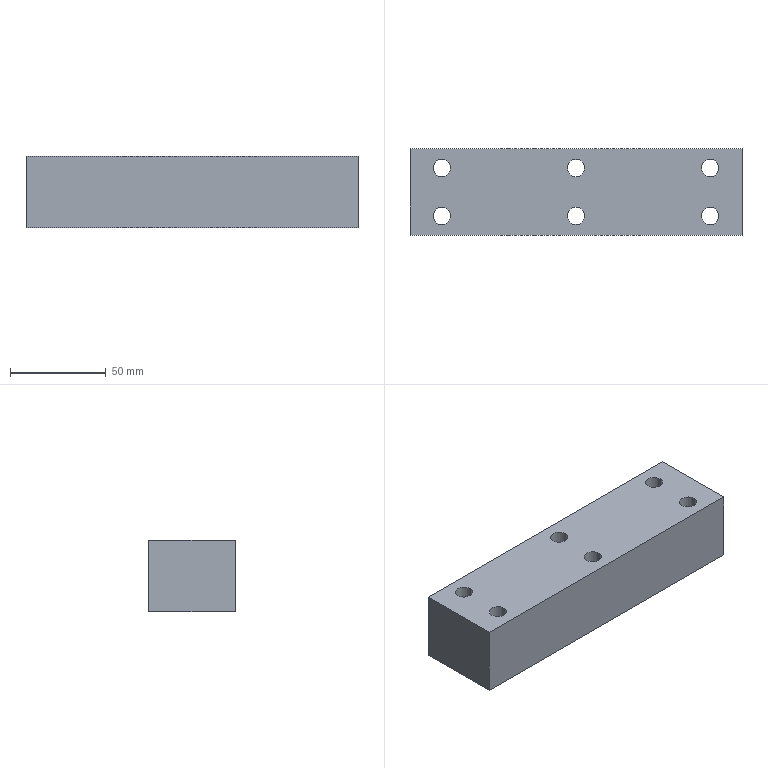Part | STEP file | 44-02-16 Press-fit Connecting Plate | 1 solid | 18 faces | box 173 x 45 x 37 mm | volume 273922 mm3 | cylinder 12 | plane 6 | commonest cylinder face diameters 9 x12
STEP:
#1=CARTESIAN_POINT('',(0.,0.,0.));
#2=DIRECTION('',(0.,0.,1.));
#3=DIRECTION('',(1.,0.,0.));
#4=AXIS2_PLACEMENT_3D('',#1,#2,#3);
#5=CARTESIAN_POINT('',(4.5,12.5,-18.5));
#6=VERTEX_POINT('',#5);
#7=CARTESIAN_POINT('',(4.5,12.5,18.5));
#8=VERTEX_POINT('',#7);
#9=CARTESIAN_POINT('',(4.5,12.5,-18.5));
#10=DIRECTION('',(0.,0.,1.));
#11=VECTOR('',#10,1.);
#12=LINE('',#9,#11);
#13=CARTESIAN_POINT('',(0.,12.5,-18.5));
#14=DIRECTION('',(0.,0.,1.));
#15=DIRECTION('',(1.,0.,0.));
#16=AXIS2_PLACEMENT_3D('',#13,#14,#15);
#17=CYLINDRICAL_SURFACE('',#16,4.5);
#18=CARTESIAN_POINT('',(6.283,0.));
#19=DIRECTION('',(0.,1.));
#20=VECTOR('',#19,1.);
#21=LINE('',#18,#20);
#22=(GEOMETRIC_REPRESENTATION_CONTEXT(2)PARAMETRIC_REPRESENTATION_CONTEXT()REPRESENTATION_CONTEXT('',''));
#23=DEFINITIONAL_REPRESENTATION('',(#21),#22);
#24=PCURVE('',#17,#23);
#25=CARTESIAN_POINT('',(0.,12.5,-18.5));
#26=DIRECTION('',(0.,0.,1.));
#27=DIRECTION('',(1.,0.,0.));
#28=AXIS2_PLACEMENT_3D('',#25,#26,#27);
#29=CYLINDRICAL_SURFACE('',#28,4.5);
#30=CARTESIAN_POINT('',(0.,0.));
#31=DIRECTION('',(0.,1.));
#32=VECTOR('',#31,1.);
#33=LINE('',#30,#32);
#34=(GEOMETRIC_REPRESENTATION_CONTEXT(2)PARAMETRIC_REPRESENTATION_CONTEXT()REPRESENTATION_CONTEXT('',''));
#35=DEFINITIONAL_REPRESENTATION('',(#33),#34);
#36=PCURVE('',#29,#35);
#37=SURFACE_CURVE('',#12,(#24,#36),.PCURVE_S1.);
#38=EDGE_CURVE('',#6,#8,#37,.T.);
#39=ORIENTED_EDGE('',*,*,#38,.T.);
#40=CARTESIAN_POINT('',(-4.5,12.5,18.5));
#41=VERTEX_POINT('',#40);
#42=CARTESIAN_POINT('',(0.,12.5,18.5));
#43=DIRECTION('',(0.,0.,1.));
#44=DIRECTION('',(1.,0.,0.));
#45=AXIS2_PLACEMENT_3D('',#42,#43,#44);
#46=CIRCLE('',#45,4.5);
#47=CARTESIAN_POINT('',(0.,37.));
#48=DIRECTION('',(1.,0.));
#49=VECTOR('',#48,1.);
#50=LINE('',#47,#49);
#51=(GEOMETRIC_REPRESENTATION_CONTEXT(2)PARAMETRIC_REPRESENTATION_CONTEXT()REPRESENTATION_CONTEXT('',''));
#52=DEFINITIONAL_REPRESENTATION('',(#50),#51);
#53=PCURVE('',#17,#52);
#54=CARTESIAN_POINT('',(86.5,-22.5,18.5));
#55=DIRECTION('',(0.,0.,1.));
#56=DIRECTION('',(1.,0.,0.));
#57=AXIS2_PLACEMENT_3D('',#54,#55,#56);
#58=PLANE('',#57);
#59=CARTESIAN_POINT('',(-86.5,35.));
#60=DIRECTION('',(1.,0.));
#61=AXIS2_PLACEMENT_2D('',#59,#60);
#62=CIRCLE('',#61,4.5);
#63=(GEOMETRIC_REPRESENTATION_CONTEXT(2)PARAMETRIC_REPRESENTATION_CONTEXT()REPRESENTATION_CONTEXT('',''));
#64=DEFINITIONAL_REPRESENTATION('',(#62),#63);
#65=PCURVE('',#58,#64);
#66=SURFACE_CURVE('',#46,(#53,#65),.PCURVE_S1.);
#67=EDGE_CURVE('',#41,#8,#66,.T.);
#68=ORIENTED_EDGE('',*,*,#67,.F.);
#69=CARTESIAN_POINT('',(-4.5,12.5,-18.5));
#70=VERTEX_POINT('',#69);
#71=CARTESIAN_POINT('',(-4.5,12.5,-18.5));
#72=DIRECTION('',(0.,0.,1.));
#73=VECTOR('',#72,1.);
#74=LINE('',#71,#73);
#75=CARTESIAN_POINT('',(3.142,0.));
#76=DIRECTION('',(0.,1.));
#77=VECTOR('',#76,1.);
#78=LINE('',#75,#77);
#79=(GEOMETRIC_REPRESENTATION_CONTEXT(2)PARAMETRIC_REPRESENTATION_CONTEXT()REPRESENTATION_CONTEXT('',''));
#80=DEFINITIONAL_REPRESENTATION('',(#78),#79);
#81=PCURVE('',#17,#80);
#82=CARTESIAN_POINT('',(3.142,0.));
#83=DIRECTION('',(0.,1.));
#84=VECTOR('',#83,1.);
#85=LINE('',#82,#84);
#86=(GEOMETRIC_REPRESENTATION_CONTEXT(2)PARAMETRIC_REPRESENTATION_CONTEXT()REPRESENTATION_CONTEXT('',''));
#87=DEFINITIONAL_REPRESENTATION('',(#85),#86);
#88=PCURVE('',#29,#87);
#89=SURFACE_CURVE('',#74,(#81,#88),.PCURVE_S1.);
#90=EDGE_CURVE('',#70,#41,#89,.T.);
#91=ORIENTED_EDGE('',*,*,#90,.F.);
#92=CARTESIAN_POINT('',(0.,12.5,-18.5));
#93=DIRECTION('',(0.,0.,1.));
#94=DIRECTION('',(1.,0.,0.));
#95=AXIS2_PLACEMENT_3D('',#92,#93,#94);
#96=CIRCLE('',#95,4.5);
#97=CARTESIAN_POINT('',(0.,0.));
#98=DIRECTION('',(1.,0.));
#99=VECTOR('',#98,1.);
#100=LINE('',#97,#99);
#101=(GEOMETRIC_REPRESENTATION_CONTEXT(2)PARAMETRIC_REPRESENTATION_CONTEXT()REPRESENTATION_CONTEXT('',''));
#102=DEFINITIONAL_REPRESENTATION('',(#100),#101);
#103=PCURVE('',#17,#102);
#104=CARTESIAN_POINT('',(86.5,-22.5,-18.5));
#105=DIRECTION('',(0.,0.,1.));
#106=DIRECTION('',(1.,0.,0.));
#107=AXIS2_PLACEMENT_3D('',#104,#105,#106);
#108=PLANE('',#107);
#109=CARTESIAN_POINT('',(-86.5,35.));
#110=DIRECTION('',(1.,0.));
#111=AXIS2_PLACEMENT_2D('',#109,#110);
#112=CIRCLE('',#111,4.5);
#113=(GEOMETRIC_REPRESENTATION_CONTEXT(2)PARAMETRIC_REPRESENTATION_CONTEXT()REPRESENTATION_CONTEXT('',''));
#114=DEFINITIONAL_REPRESENTATION('',(#112),#113);
#115=PCURVE('',#108,#114);
#116=SURFACE_CURVE('',#96,(#103,#115),.PCURVE_S1.);
#117=EDGE_CURVE('',#70,#6,#116,.T.);
#118=ORIENTED_EDGE('',*,*,#117,.T.);
#119=EDGE_LOOP('',(#39,#68,#91,#118));
#120=FACE_BOUND('',#119,.F.);
#121=ADVANCED_FACE('',(#120),#17,.F.);
#122=CARTESIAN_POINT('',(4.5,-12.5,-18.5));
#123=VERTEX_POINT('',#122);
#124=CARTESIAN_POINT('',(4.5,-12.5,18.5));
#125=VERTEX_POINT('',#124);
#126=CARTESIAN_POINT('',(4.5,-12.5,-18.5));
#127=DIRECTION('',(0.,0.,1.));
#128=VECTOR('',#127,1.);
#129=LINE('',#126,#128);
#130=CARTESIAN_POINT('',(0.,-12.5,-18.5));
#131=DIRECTION('',(0.,0.,1.));
#132=DIRECTION('',(1.,0.,0.));
#133=AXIS2_PLACEMENT_3D('',#130,#131,#132);
#134=CYLINDRICAL_SURFACE('',#133,4.5);
#135=CARTESIAN_POINT('',(6.283,0.));
#136=DIRECTION('',(0.,1.));
#137=VECTOR('',#136,1.);
#138=LINE('',#135,#137);
#139=(GEOMETRIC_REPRESENTATION_CONTEXT(2)PARAMETRIC_REPRESENTATION_CONTEXT()REPRESENTATION_CONTEXT('',''));
#140=DEFINITIONAL_REPRESENTATION('',(#138),#139);
#141=PCURVE('',#134,#140);
#142=CARTESIAN_POINT('',(0.,-12.5,-18.5));
#143=DIRECTION('',(0.,0.,1.));
#144=DIRECTION('',(1.,0.,0.));
#145=AXIS2_PLACEMENT_3D('',#142,#143,#144);
#146=CYLINDRICAL_SURFACE('',#145,4.5);
#147=CARTESIAN_POINT('',(0.,0.));
#148=DIRECTION('',(0.,1.));
#149=VECTOR('',#148,1.);
#150=LINE('',#147,#149);
#151=(GEOMETRIC_REPRESENTATION_CONTEXT(2)PARAMETRIC_REPRESENTATION_CONTEXT()REPRESENTATION_CONTEXT('',''));
#152=DEFINITIONAL_REPRESENTATION('',(#150),#151);
#153=PCURVE('',#146,#152);
#154=SURFACE_CURVE('',#129,(#141,#153),.PCURVE_S1.);
#155=EDGE_CURVE('',#123,#125,#154,.T.);
#156=ORIENTED_EDGE('',*,*,#155,.T.);
#157=CARTESIAN_POINT('',(-4.5,-12.5,18.5));
#158=VERTEX_POINT('',#157);
#159=CARTESIAN_POINT('',(0.,-12.5,18.5));
#160=DIRECTION('',(0.,0.,1.));
#161=DIRECTION('',(1.,0.,0.));
#162=AXIS2_PLACEMENT_3D('',#159,#160,#161);
#163=CIRCLE('',#162,4.5);
#164=CARTESIAN_POINT('',(0.,37.));
#165=DIRECTION('',(1.,0.));
#166=VECTOR('',#165,1.);
#167=LINE('',#164,#166);
#168=(GEOMETRIC_REPRESENTATION_CONTEXT(2)PARAMETRIC_REPRESENTATION_CONTEXT()REPRESENTATION_CONTEXT('',''));
#169=DEFINITIONAL_REPRESENTATION('',(#167),#168);
#170=PCURVE('',#134,#169);
#171=CARTESIAN_POINT('',(-86.5,10.));
#172=DIRECTION('',(1.,0.));
#173=AXIS2_PLACEMENT_2D('',#171,#172);
#174=CIRCLE('',#173,4.5);
#175=(GEOMETRIC_REPRESENTATION_CONTEXT(2)PARAMETRIC_REPRESENTATION_CONTEXT()REPRESENTATION_CONTEXT('',''));
#176=DEFINITIONAL_REPRESENTATION('',(#174),#175);
#177=PCURVE('',#58,#176);
#178=SURFACE_CURVE('',#163,(#170,#177),.PCURVE_S1.);
#179=EDGE_CURVE('',#158,#125,#178,.T.);
#180=ORIENTED_EDGE('',*,*,#179,.F.);
#181=CARTESIAN_POINT('',(-4.5,-12.5,-18.5));
#182=VERTEX_POINT('',#181);
#183=CARTESIAN_POINT('',(-4.5,-12.5,-18.5));
#184=DIRECTION('',(0.,0.,1.));
#185=VECTOR('',#184,1.);
#186=LINE('',#183,#185);
#187=CARTESIAN_POINT('',(3.142,0.));
#188=DIRECTION('',(0.,1.));
#189=VECTOR('',#188,1.);
#190=LINE('',#187,#189);
#191=(GEOMETRIC_REPRESENTATION_CONTEXT(2)PARAMETRIC_REPRESENTATION_CONTEXT()REPRESENTATION_CONTEXT('',''));
#192=DEFINITIONAL_REPRESENTATION('',(#190),#191);
#193=PCURVE('',#134,#192);
#194=CARTESIAN_POINT('',(3.142,0.));
#195=DIRECTION('',(0.,1.));
#196=VECTOR('',#195,1.);
#197=LINE('',#194,#196);
#198=(GEOMETRIC_REPRESENTATION_CONTEXT(2)PARAMETRIC_REPRESENTATION_CONTEXT()REPRESENTATION_CONTEXT('',''));
#199=DEFINITIONAL_REPRESENTATION('',(#197),#198);
#200=PCURVE('',#146,#199);
#201=SURFACE_CURVE('',#186,(#193,#200),.PCURVE_S1.);
#202=EDGE_CURVE('',#182,#158,#201,.T.);
#203=ORIENTED_EDGE('',*,*,#202,.F.);
#204=CARTESIAN_POINT('',(0.,-12.5,-18.5));
#205=DIRECTION('',(0.,0.,1.));
#206=DIRECTION('',(1.,0.,0.));
#207=AXIS2_PLACEMENT_3D('',#204,#205,#206);
#208=CIRCLE('',#207,4.5);
#209=CARTESIAN_POINT('',(0.,0.));
#210=DIRECTION('',(1.,0.));
#211=VECTOR('',#210,1.);
#212=LINE('',#209,#211);
#213=(GEOMETRIC_REPRESENTATION_CONTEXT(2)PARAMETRIC_REPRESENTATION_CONTEXT()REPRESENTATION_CONTEXT('',''));
#214=DEFINITIONAL_REPRESENTATION('',(#212),#213);
#215=PCURVE('',#134,#214);
#216=CARTESIAN_POINT('',(-86.5,10.));
#217=DIRECTION('',(1.,0.));
#218=AXIS2_PLACEMENT_2D('',#216,#217);
#219=CIRCLE('',#218,4.5);
#220=(GEOMETRIC_REPRESENTATION_CONTEXT(2)PARAMETRIC_REPRESENTATION_CONTEXT()REPRESENTATION_CONTEXT('',''));
#221=DEFINITIONAL_REPRESENTATION('',(#219),#220);
#222=PCURVE('',#108,#221);
#223=SURFACE_CURVE('',#208,(#215,#222),.PCURVE_S1.);
#224=EDGE_CURVE('',#182,#123,#223,.T.);
#225=ORIENTED_EDGE('',*,*,#224,.T.);
#226=EDGE_LOOP('',(#156,#180,#203,#225));
#227=FACE_BOUND('',#226,.F.);
#228=ADVANCED_FACE('',(#227),#134,.F.);
#229=CARTESIAN_POINT('',(74.5,12.5,-18.5));
#230=VERTEX_POINT('',#229);
#231=CARTESIAN_POINT('',(74.5,12.5,18.5));
#232=VERTEX_POINT('',#231);
#233=CARTESIAN_POINT('',(74.5,12.5,-18.5));
#234=DIRECTION('',(0.,0.,1.));
#235=VECTOR('',#234,1.);
#236=LINE('',#233,#235);
#237=CARTESIAN_POINT('',(70.,12.5,-18.5));
#238=DIRECTION('',(0.,0.,1.));
#239=DIRECTION('',(1.,0.,0.));
#240=AXIS2_PLACEMENT_3D('',#237,#238,#239);
#241=CYLINDRICAL_SURFACE('',#240,4.5);
#242=CARTESIAN_POINT('',(6.283,0.));
#243=DIRECTION('',(0.,1.));
#244=VECTOR('',#243,1.);
#245=LINE('',#242,#244);
#246=(GEOMETRIC_REPRESENTATION_CONTEXT(2)PARAMETRIC_REPRESENTATION_CONTEXT()REPRESENTATION_CONTEXT('',''));
#247=DEFINITIONAL_REPRESENTATION('',(#245),#246);
#248=PCURVE('',#241,#247);
#249=CARTESIAN_POINT('',(70.,12.5,-18.5));
#250=DIRECTION('',(0.,0.,1.));
#251=DIRECTION('',(1.,0.,0.));
#252=AXIS2_PLACEMENT_3D('',#249,#250,#251);
#253=CYLINDRICAL_SURFACE('',#252,4.5);
#254=CARTESIAN_POINT('',(0.,0.));
#255=DIRECTION('',(0.,1.));
#256=VECTOR('',#255,1.);
#257=LINE('',#254,#256);
#258=(GEOMETRIC_REPRESENTATION_CONTEXT(2)PARAMETRIC_REPRESENTATION_CONTEXT()REPRESENTATION_CONTEXT('',''));
#259=DEFINITIONAL_REPRESENTATION('',(#257),#258);
#260=PCURVE('',#253,#259);
#261=SURFACE_CURVE('',#236,(#248,#260),.PCURVE_S1.);
#262=EDGE_CURVE('',#230,#232,#261,.T.);
#263=ORIENTED_EDGE('',*,*,#262,.T.);
#264=CARTESIAN_POINT('',(65.5,12.5,18.5));
#265=VERTEX_POINT('',#264);
#266=CARTESIAN_POINT('',(70.,12.5,18.5));
#267=DIRECTION('',(0.,0.,1.));
#268=DIRECTION('',(1.,0.,0.));
#269=AXIS2_PLACEMENT_3D('',#266,#267,#268);
#270=CIRCLE('',#269,4.5);
#271=CARTESIAN_POINT('',(0.,37.));
#272=DIRECTION('',(1.,0.));
#273=VECTOR('',#272,1.);
#274=LINE('',#271,#273);
#275=(GEOMETRIC_REPRESENTATION_CONTEXT(2)PARAMETRIC_REPRESENTATION_CONTEXT()REPRESENTATION_CONTEXT('',''));
#276=DEFINITIONAL_REPRESENTATION('',(#274),#275);
#277=PCURVE('',#241,#276);
#278=CARTESIAN_POINT('',(-16.5,35.));
#279=DIRECTION('',(1.,0.));
#280=AXIS2_PLACEMENT_2D('',#278,#279);
#281=CIRCLE('',#280,4.5);
#282=(GEOMETRIC_REPRESENTATION_CONTEXT(2)PARAMETRIC_REPRESENTATION_CONTEXT()REPRESENTATION_CONTEXT('',''));
#283=DEFINITIONAL_REPRESENTATION('',(#281),#282);
#284=PCURVE('',#58,#283);
#285=SURFACE_CURVE('',#270,(#277,#284),.PCURVE_S1.);
#286=EDGE_CURVE('',#265,#232,#285,.T.);
#287=ORIENTED_EDGE('',*,*,#286,.F.);
#288=CARTESIAN_POINT('',(65.5,12.5,-18.5));
#289=VERTEX_POINT('',#288);
#290=CARTESIAN_POINT('',(65.5,12.5,-18.5));
#291=DIRECTION('',(0.,0.,1.));
#292=VECTOR('',#291,1.);
#293=LINE('',#290,#292);
#294=CARTESIAN_POINT('',(3.142,0.));
#295=DIRECTION('',(0.,1.));
#296=VECTOR('',#295,1.);
#297=LINE('',#294,#296);
#298=(GEOMETRIC_REPRESENTATION_CONTEXT(2)PARAMETRIC_REPRESENTATION_CONTEXT()REPRESENTATION_CONTEXT('',''));
#299=DEFINITIONAL_REPRESENTATION('',(#297),#298);
#300=PCURVE('',#241,#299);
#301=CARTESIAN_POINT('',(3.142,0.));
#302=DIRECTION('',(0.,1.));
#303=VECTOR('',#302,1.);
#304=LINE('',#301,#303);
#305=(GEOMETRIC_REPRESENTATION_CONTEXT(2)PARAMETRIC_REPRESENTATION_CONTEXT()REPRESENTATION_CONTEXT('',''));
#306=DEFINITIONAL_REPRESENTATION('',(#304),#305);
#307=PCURVE('',#253,#306);
#308=SURFACE_CURVE('',#293,(#300,#307),.PCURVE_S1.);
#309=EDGE_CURVE('',#289,#265,#308,.T.);
#310=ORIENTED_EDGE('',*,*,#309,.F.);
#311=CARTESIAN_POINT('',(70.,12.5,-18.5));
#312=DIRECTION('',(0.,0.,1.));
#313=DIRECTION('',(1.,0.,0.));
#314=AXIS2_PLACEMENT_3D('',#311,#312,#313);
#315=CIRCLE('',#314,4.5);
#316=CARTESIAN_POINT('',(0.,0.));
#317=DIRECTION('',(1.,0.));
#318=VECTOR('',#317,1.);
#319=LINE('',#316,#318);
#320=(GEOMETRIC_REPRESENTATION_CONTEXT(2)PARAMETRIC_REPRESENTATION_CONTEXT()REPRESENTATION_CONTEXT('',''));
#321=DEFINITIONAL_REPRESENTATION('',(#319),#320);
#322=PCURVE('',#241,#321);
#323=CARTESIAN_POINT('',(-16.5,35.));
#324=DIRECTION('',(1.,0.));
#325=AXIS2_PLACEMENT_2D('',#323,#324);
#326=CIRCLE('',#325,4.5);
#327=(GEOMETRIC_REPRESENTATION_CONTEXT(2)PARAMETRIC_REPRESENTATION_CONTEXT()REPRESENTATION_CONTEXT('',''));
#328=DEFINITIONAL_REPRESENTATION('',(#326),#327);
#329=PCURVE('',#108,#328);
#330=SURFACE_CURVE('',#315,(#322,#329),.PCURVE_S1.);
#331=EDGE_CURVE('',#289,#230,#330,.T.);
#332=ORIENTED_EDGE('',*,*,#331,.T.);
#333=EDGE_LOOP('',(#263,#287,#310,#332));
#334=FACE_BOUND('',#333,.F.);
#335=ADVANCED_FACE('',(#334),#241,.F.);
#336=CARTESIAN_POINT('',(74.5,-12.5,-18.5));
#337=VERTEX_POINT('',#336);
#338=CARTESIAN_POINT('',(74.5,-12.5,18.5));
#339=VERTEX_POINT('',#338);
#340=CARTESIAN_POINT('',(74.5,-12.5,-18.5));
#341=DIRECTION('',(0.,0.,1.));
#342=VECTOR('',#341,1.);
#343=LINE('',#340,#342);
#344=CARTESIAN_POINT('',(70.,-12.5,-18.5));
#345=DIRECTION('',(0.,0.,1.));
#346=DIRECTION('',(1.,0.,0.));
#347=AXIS2_PLACEMENT_3D('',#344,#345,#346);
#348=CYLINDRICAL_SURFACE('',#347,4.5);
#349=CARTESIAN_POINT('',(6.283,0.));
#350=DIRECTION('',(0.,1.));
#351=VECTOR('',#350,1.);
#352=LINE('',#349,#351);
#353=(GEOMETRIC_REPRESENTATION_CONTEXT(2)PARAMETRIC_REPRESENTATION_CONTEXT()REPRESENTATION_CONTEXT('',''));
#354=DEFINITIONAL_REPRESENTATION('',(#352),#353);
#355=PCURVE('',#348,#354);
#356=CARTESIAN_POINT('',(70.,-12.5,-18.5));
#357=DIRECTION('',(0.,0.,1.));
#358=DIRECTION('',(1.,0.,0.));
#359=AXIS2_PLACEMENT_3D('',#356,#357,#358);
#360=CYLINDRICAL_SURFACE('',#359,4.5);
#361=CARTESIAN_POINT('',(0.,0.));
#362=DIRECTION('',(0.,1.));
#363=VECTOR('',#362,1.);
#364=LINE('',#361,#363);
#365=(GEOMETRIC_REPRESENTATION_CONTEXT(2)PARAMETRIC_REPRESENTATION_CONTEXT()REPRESENTATION_CONTEXT('',''));
#366=DEFINITIONAL_REPRESENTATION('',(#364),#365);
#367=PCURVE('',#360,#366);
#368=SURFACE_CURVE('',#343,(#355,#367),.PCURVE_S1.);
#369=EDGE_CURVE('',#337,#339,#368,.T.);
#370=ORIENTED_EDGE('',*,*,#369,.T.);
#371=CARTESIAN_POINT('',(65.5,-12.5,18.5));
#372=VERTEX_POINT('',#371);
#373=CARTESIAN_POINT('',(70.,-12.5,18.5));
#374=DIRECTION('',(0.,0.,1.));
#375=DIRECTION('',(1.,0.,0.));
#376=AXIS2_PLACEMENT_3D('',#373,#374,#375);
#377=CIRCLE('',#376,4.5);
#378=CARTESIAN_POINT('',(0.,37.));
#379=DIRECTION('',(1.,0.));
#380=VECTOR('',#379,1.);
#381=LINE('',#378,#380);
#382=(GEOMETRIC_REPRESENTATION_CONTEXT(2)PARAMETRIC_REPRESENTATION_CONTEXT()REPRESENTATION_CONTEXT('',''));
#383=DEFINITIONAL_REPRESENTATION('',(#381),#382);
#384=PCURVE('',#348,#383);
#385=CARTESIAN_POINT('',(-16.5,10.));
#386=DIRECTION('',(1.,0.));
#387=AXIS2_PLACEMENT_2D('',#385,#386);
#388=CIRCLE('',#387,4.5);
#389=(GEOMETRIC_REPRESENTATION_CONTEXT(2)PARAMETRIC_REPRESENTATION_CONTEXT()REPRESENTATION_CONTEXT('',''));
#390=DEFINITIONAL_REPRESENTATION('',(#388),#389);
#391=PCURVE('',#58,#390);
#392=SURFACE_CURVE('',#377,(#384,#391),.PCURVE_S1.);
#393=EDGE_CURVE('',#372,#339,#392,.T.);
#394=ORIENTED_EDGE('',*,*,#393,.F.);
#395=CARTESIAN_POINT('',(65.5,-12.5,-18.5));
#396=VERTEX_POINT('',#395);
#397=CARTESIAN_POINT('',(65.5,-12.5,-18.5));
#398=DIRECTION('',(0.,0.,1.));
#399=VECTOR('',#398,1.);
#400=LINE('',#397,#399);
#401=CARTESIAN_POINT('',(3.142,0.));
#402=DIRECTION('',(0.,1.));
#403=VECTOR('',#402,1.);
#404=LINE('',#401,#403);
#405=(GEOMETRIC_REPRESENTATION_CONTEXT(2)PARAMETRIC_REPRESENTATION_CONTEXT()REPRESENTATION_CONTEXT('',''));
#406=DEFINITIONAL_REPRESENTATION('',(#404),#405);
#407=PCURVE('',#348,#406);
#408=CARTESIAN_POINT('',(3.142,0.));
#409=DIRECTION('',(0.,1.));
#410=VECTOR('',#409,1.);
#411=LINE('',#408,#410);
#412=(GEOMETRIC_REPRESENTATION_CONTEXT(2)PARAMETRIC_REPRESENTATION_CONTEXT()REPRESENTATION_CONTEXT('',''));
#413=DEFINITIONAL_REPRESENTATION('',(#411),#412);
#414=PCURVE('',#360,#413);
#415=SURFACE_CURVE('',#400,(#407,#414),.PCURVE_S1.);
#416=EDGE_CURVE('',#396,#372,#415,.T.);
#417=ORIENTED_EDGE('',*,*,#416,.F.);
#418=CARTESIAN_POINT('',(70.,-12.5,-18.5));
#419=DIRECTION('',(0.,0.,1.));
#420=DIRECTION('',(1.,0.,0.));
#421=AXIS2_PLACEMENT_3D('',#418,#419,#420);
#422=CIRCLE('',#421,4.5);
#423=CARTESIAN_POINT('',(0.,0.));
#424=DIRECTION('',(1.,0.));
#425=VECTOR('',#424,1.);
#426=LINE('',#423,#425);
#427=(GEOMETRIC_REPRESENTATION_CONTEXT(2)PARAMETRIC_REPRESENTATION_CONTEXT()REPRESENTATION_CONTEXT('',''));
#428=DEFINITIONAL_REPRESENTATION('',(#426),#427);
#429=PCURVE('',#348,#428);
#430=CARTESIAN_POINT('',(-16.5,10.));
#431=DIRECTION('',(1.,0.));
#432=AXIS2_PLACEMENT_2D('',#430,#431);
#433=CIRCLE('',#432,4.5);
#434=(GEOMETRIC_REPRESENTATION_CONTEXT(2)PARAMETRIC_REPRESENTATION_CONTEXT()REPRESENTATION_CONTEXT('',''));
#435=DEFINITIONAL_REPRESENTATION('',(#433),#434);
#436=PCURVE('',#108,#435);
#437=SURFACE_CURVE('',#422,(#429,#436),.PCURVE_S1.);
#438=EDGE_CURVE('',#396,#337,#437,.T.);
#439=ORIENTED_EDGE('',*,*,#438,.T.);
#440=EDGE_LOOP('',(#370,#394,#417,#439));
#441=FACE_BOUND('',#440,.F.);
#442=ADVANCED_FACE('',(#441),#348,.F.);
#443=CARTESIAN_POINT('',(-65.5,-12.5,-18.5));
#444=VERTEX_POINT('',#443);
#445=CARTESIAN_POINT('',(-65.5,-12.5,18.5));
#446=VERTEX_POINT('',#445);
#447=CARTESIAN_POINT('',(-65.5,-12.5,-18.5));
#448=DIRECTION('',(0.,0.,1.));
#449=VECTOR('',#448,1.);
#450=LINE('',#447,#449);
#451=CARTESIAN_POINT('',(-70.,-12.5,-18.5));
#452=DIRECTION('',(0.,0.,1.));
#453=DIRECTION('',(1.,0.,0.));
#454=AXIS2_PLACEMENT_3D('',#451,#452,#453);
#455=CYLINDRICAL_SURFACE('',#454,4.5);
#456=CARTESIAN_POINT('',(6.283,0.));
#457=DIRECTION('',(0.,1.));
#458=VECTOR('',#457,1.);
#459=LINE('',#456,#458);
#460=(GEOMETRIC_REPRESENTATION_CONTEXT(2)PARAMETRIC_REPRESENTATION_CONTEXT()REPRESENTATION_CONTEXT('',''));
#461=DEFINITIONAL_REPRESENTATION('',(#459),#460);
#462=PCURVE('',#455,#461);
#463=CARTESIAN_POINT('',(-70.,-12.5,-18.5));
#464=DIRECTION('',(0.,0.,1.));
#465=DIRECTION('',(1.,0.,0.));
#466=AXIS2_PLACEMENT_3D('',#463,#464,#465);
#467=CYLINDRICAL_SURFACE('',#466,4.5);
#468=CARTESIAN_POINT('',(0.,0.));
#469=DIRECTION('',(0.,1.));
#470=VECTOR('',#469,1.);
#471=LINE('',#468,#470);
#472=(GEOMETRIC_REPRESENTATION_CONTEXT(2)PARAMETRIC_REPRESENTATION_CONTEXT()REPRESENTATION_CONTEXT('',''));
#473=DEFINITIONAL_REPRESENTATION('',(#471),#472);
#474=PCURVE('',#467,#473);
#475=SURFACE_CURVE('',#450,(#462,#474),.PCURVE_S1.);
#476=EDGE_CURVE('',#444,#446,#475,.T.);
#477=ORIENTED_EDGE('',*,*,#476,.T.);
#478=CARTESIAN_POINT('',(-74.5,-12.5,18.5));
#479=VERTEX_POINT('',#478);
#480=CARTESIAN_POINT('',(-70.,-12.5,18.5));
#481=DIRECTION('',(0.,0.,1.));
#482=DIRECTION('',(1.,0.,0.));
#483=AXIS2_PLACEMENT_3D('',#480,#481,#482);
#484=CIRCLE('',#483,4.5);
#485=CARTESIAN_POINT('',(0.,37.));
#486=DIRECTION('',(1.,0.));
#487=VECTOR('',#486,1.);
#488=LINE('',#485,#487);
#489=(GEOMETRIC_REPRESENTATION_CONTEXT(2)PARAMETRIC_REPRESENTATION_CONTEXT()REPRESENTATION_CONTEXT('',''));
#490=DEFINITIONAL_REPRESENTATION('',(#488),#489);
#491=PCURVE('',#455,#490);
#492=CARTESIAN_POINT('',(-156.5,10.));
#493=DIRECTION('',(1.,0.));
#494=AXIS2_PLACEMENT_2D('',#492,#493);
#495=CIRCLE('',#494,4.5);
#496=(GEOMETRIC_REPRESENTATION_CONTEXT(2)PARAMETRIC_REPRESENTATION_CONTEXT()REPRESENTATION_CONTEXT('',''));
#497=DEFINITIONAL_REPRESENTATION('',(#495),#496);
#498=PCURVE('',#58,#497);
#499=SURFACE_CURVE('',#484,(#491,#498),.PCURVE_S1.);
#500=EDGE_CURVE('',#479,#446,#499,.T.);
#501=ORIENTED_EDGE('',*,*,#500,.F.);
#502=CARTESIAN_POINT('',(-74.5,-12.5,-18.5));
#503=VERTEX_POINT('',#502);
#504=CARTESIAN_POINT('',(-74.5,-12.5,-18.5));
#505=DIRECTION('',(0.,0.,1.));
#506=VECTOR('',#505,1.);
#507=LINE('',#504,#506);
#508=CARTESIAN_POINT('',(3.142,0.));
#509=DIRECTION('',(0.,1.));
#510=VECTOR('',#509,1.);
#511=LINE('',#508,#510);
#512=(GEOMETRIC_REPRESENTATION_CONTEXT(2)PARAMETRIC_REPRESENTATION_CONTEXT()REPRESENTATION_CONTEXT('',''));
#513=DEFINITIONAL_REPRESENTATION('',(#511),#512);
#514=PCURVE('',#455,#513);
#515=CARTESIAN_POINT('',(3.142,0.));
#516=DIRECTION('',(0.,1.));
#517=VECTOR('',#516,1.);
#518=LINE('',#515,#517);
#519=(GEOMETRIC_REPRESENTATION_CONTEXT(2)PARAMETRIC_REPRESENTATION_CONTEXT()REPRESENTATION_CONTEXT('',''));
#520=DEFINITIONAL_REPRESENTATION('',(#518),#519);
#521=PCURVE('',#467,#520);
#522=SURFACE_CURVE('',#507,(#514,#521),.PCURVE_S1.);
#523=EDGE_CURVE('',#503,#479,#522,.T.);
#524=ORIENTED_EDGE('',*,*,#523,.F.);
#525=CARTESIAN_POINT('',(-70.,-12.5,-18.5));
#526=DIRECTION('',(0.,0.,1.));
#527=DIRECTION('',(1.,0.,0.));
#528=AXIS2_PLACEMENT_3D('',#525,#526,#527);
#529=CIRCLE('',#528,4.5);
#530=CARTESIAN_POINT('',(0.,0.));
#531=DIRECTION('',(1.,0.));
#532=VECTOR('',#531,1.);
#533=LINE('',#530,#532);
#534=(GEOMETRIC_REPRESENTATION_CONTEXT(2)PARAMETRIC_REPRESENTATION_CONTEXT()REPRESENTATION_CONTEXT('',''));
#535=DEFINITIONAL_REPRESENTATION('',(#533),#534);
#536=PCURVE('',#455,#535);
#537=CARTESIAN_POINT('',(-156.5,10.));
#538=DIRECTION('',(1.,0.));
#539=AXIS2_PLACEMENT_2D('',#537,#538);
#540=CIRCLE('',#539,4.5);
#541=(GEOMETRIC_REPRESENTATION_CONTEXT(2)PARAMETRIC_REPRESENTATION_CONTEXT()REPRESENTATION_CONTEXT('',''));
#542=DEFINITIONAL_REPRESENTATION('',(#540),#541);
#543=PCURVE('',#108,#542);
#544=SURFACE_CURVE('',#529,(#536,#543),.PCURVE_S1.);
#545=EDGE_CURVE('',#503,#444,#544,.T.);
#546=ORIENTED_EDGE('',*,*,#545,.T.);
#547=EDGE_LOOP('',(#477,#501,#524,#546));
#548=FACE_BOUND('',#547,.F.);
#549=ADVANCED_FACE('',(#548),#455,.F.);
#550=CARTESIAN_POINT('',(-65.5,12.5,-18.5));
#551=VERTEX_POINT('',#550);
#552=CARTESIAN_POINT('',(-65.5,12.5,18.5));
#553=VERTEX_POINT('',#552);
#554=CARTESIAN_POINT('',(-65.5,12.5,-18.5));
#555=DIRECTION('',(0.,0.,1.));
#556=VECTOR('',#555,1.);
#557=LINE('',#554,#556);
#558=CARTESIAN_POINT('',(-70.,12.5,-18.5));
#559=DIRECTION('',(0.,0.,1.));
#560=DIRECTION('',(1.,0.,0.));
#561=AXIS2_PLACEMENT_3D('',#558,#559,#560);
#562=CYLINDRICAL_SURFACE('',#561,4.5);
#563=CARTESIAN_POINT('',(6.283,0.));
#564=DIRECTION('',(0.,1.));
#565=VECTOR('',#564,1.);
#566=LINE('',#563,#565);
#567=(GEOMETRIC_REPRESENTATION_CONTEXT(2)PARAMETRIC_REPRESENTATION_CONTEXT()REPRESENTATION_CONTEXT('',''));
#568=DEFINITIONAL_REPRESENTATION('',(#566),#567);
#569=PCURVE('',#562,#568);
#570=CARTESIAN_POINT('',(-70.,12.5,-18.5));
#571=DIRECTION('',(0.,0.,1.));
#572=DIRECTION('',(1.,0.,0.));
#573=AXIS2_PLACEMENT_3D('',#570,#571,#572);
#574=CYLINDRICAL_SURFACE('',#573,4.5);
#575=CARTESIAN_POINT('',(0.,0.));
#576=DIRECTION('',(0.,1.));
#577=VECTOR('',#576,1.);
#578=LINE('',#575,#577);
#579=(GEOMETRIC_REPRESENTATION_CONTEXT(2)PARAMETRIC_REPRESENTATION_CONTEXT()REPRESENTATION_CONTEXT('',''));
#580=DEFINITIONAL_REPRESENTATION('',(#578),#579);
#581=PCURVE('',#574,#580);
#582=SURFACE_CURVE('',#557,(#569,#581),.PCURVE_S1.);
#583=EDGE_CURVE('',#551,#553,#582,.T.);
#584=ORIENTED_EDGE('',*,*,#583,.T.);
#585=CARTESIAN_POINT('',(-74.5,12.5,18.5));
#586=VERTEX_POINT('',#585);
#587=CARTESIAN_POINT('',(-70.,12.5,18.5));
#588=DIRECTION('',(0.,0.,1.));
#589=DIRECTION('',(1.,0.,0.));
#590=AXIS2_PLACEMENT_3D('',#587,#588,#589);
#591=CIRCLE('',#590,4.5);
#592=CARTESIAN_POINT('',(0.,37.));
#593=DIRECTION('',(1.,0.));
#594=VECTOR('',#593,1.);
#595=LINE('',#592,#594);
#596=(GEOMETRIC_REPRESENTATION_CONTEXT(2)PARAMETRIC_REPRESENTATION_CONTEXT()REPRESENTATION_CONTEXT('',''));
#597=DEFINITIONAL_REPRESENTATION('',(#595),#596);
#598=PCURVE('',#562,#597);
#599=CARTESIAN_POINT('',(-156.5,35.));
#600=DIRECTION('',(1.,0.));
#601=AXIS2_PLACEMENT_2D('',#599,#600);
#602=CIRCLE('',#601,4.5);
#603=(GEOMETRIC_REPRESENTATION_CONTEXT(2)PARAMETRIC_REPRESENTATION_CONTEXT()REPRESENTATION_CONTEXT('',''));
#604=DEFINITIONAL_REPRESENTATION('',(#602),#603);
#605=PCURVE('',#58,#604);
#606=SURFACE_CURVE('',#591,(#598,#605),.PCURVE_S1.);
#607=EDGE_CURVE('',#586,#553,#606,.T.);
#608=ORIENTED_EDGE('',*,*,#607,.F.);
#609=CARTESIAN_POINT('',(-74.5,12.5,-18.5));
#610=VERTEX_POINT('',#609);
#611=CARTESIAN_POINT('',(-74.5,12.5,-18.5));
#612=DIRECTION('',(0.,0.,1.));
#613=VECTOR('',#612,1.);
#614=LINE('',#611,#613);
#615=CARTESIAN_POINT('',(3.142,0.));
#616=DIRECTION('',(0.,1.));
#617=VECTOR('',#616,1.);
#618=LINE('',#615,#617);
#619=(GEOMETRIC_REPRESENTATION_CONTEXT(2)PARAMETRIC_REPRESENTATION_CONTEXT()REPRESENTATION_CONTEXT('',''));
#620=DEFINITIONAL_REPRESENTATION('',(#618),#619);
#621=PCURVE('',#562,#620);
#622=CARTESIAN_POINT('',(3.142,0.));
#623=DIRECTION('',(0.,1.));
#624=VECTOR('',#623,1.);
#625=LINE('',#622,#624);
#626=(GEOMETRIC_REPRESENTATION_CONTEXT(2)PARAMETRIC_REPRESENTATION_CONTEXT()REPRESENTATION_CONTEXT('',''));
#627=DEFINITIONAL_REPRESENTATION('',(#625),#626);
#628=PCURVE('',#574,#627);
#629=SURFACE_CURVE('',#614,(#621,#628),.PCURVE_S1.);
#630=EDGE_CURVE('',#610,#586,#629,.T.);
#631=ORIENTED_EDGE('',*,*,#630,.F.);
#632=CARTESIAN_POINT('',(-70.,12.5,-18.5));
#633=DIRECTION('',(0.,0.,1.));
#634=DIRECTION('',(1.,0.,0.));
#635=AXIS2_PLACEMENT_3D('',#632,#633,#634);
#636=CIRCLE('',#635,4.5);
#637=CARTESIAN_POINT('',(0.,0.));
#638=DIRECTION('',(1.,0.));
#639=VECTOR('',#638,1.);
#640=LINE('',#637,#639);
#641=(GEOMETRIC_REPRESENTATION_CONTEXT(2)PARAMETRIC_REPRESENTATION_CONTEXT()REPRESENTATION_CONTEXT('',''));
#642=DEFINITIONAL_REPRESENTATION('',(#640),#641);
#643=PCURVE('',#562,#642);
#644=CARTESIAN_POINT('',(-156.5,35.));
#645=DIRECTION('',(1.,0.));
#646=AXIS2_PLACEMENT_2D('',#644,#645);
#647=CIRCLE('',#646,4.5);
#648=(GEOMETRIC_REPRESENTATION_CONTEXT(2)PARAMETRIC_REPRESENTATION_CONTEXT()REPRESENTATION_CONTEXT('',''));
#649=DEFINITIONAL_REPRESENTATION('',(#647),#648);
#650=PCURVE('',#108,#649);
#651=SURFACE_CURVE('',#636,(#643,#650),.PCURVE_S1.);
#652=EDGE_CURVE('',#610,#551,#651,.T.);
#653=ORIENTED_EDGE('',*,*,#652,.T.);
#654=EDGE_LOOP('',(#584,#608,#631,#653));
#655=FACE_BOUND('',#654,.F.);
#656=ADVANCED_FACE('',(#655),#562,.F.);
#657=CARTESIAN_POINT('',(86.5,-22.5,-18.5));
#658=VERTEX_POINT('',#657);
#659=CARTESIAN_POINT('',(86.5,22.5,-18.5));
#660=VERTEX_POINT('',#659);
#661=CARTESIAN_POINT('',(86.5,22.5,-18.5));
#662=DIRECTION('',(0.,1.,0.));
#663=VECTOR('',#662,1.);
#664=LINE('',#661,#663);
#665=CARTESIAN_POINT('',(86.5,22.5,18.5));
#666=DIRECTION('',(-1.,0.,0.));
#667=DIRECTION('',(0.,0.,1.));
#668=AXIS2_PLACEMENT_3D('',#665,#666,#667);
#669=PLANE('',#668);
#670=CARTESIAN_POINT('',(-37.,0.));
#671=DIRECTION('',(0.,1.));
#672=VECTOR('',#671,1.);
#673=LINE('',#670,#672);
#674=(GEOMETRIC_REPRESENTATION_CONTEXT(2)PARAMETRIC_REPRESENTATION_CONTEXT()REPRESENTATION_CONTEXT('',''));
#675=DEFINITIONAL_REPRESENTATION('',(#673),#674);
#676=PCURVE('',#669,#675);
#677=CARTESIAN_POINT('',(0.,45.));
#678=DIRECTION('',(0.,1.));
#679=VECTOR('',#678,1.);
#680=LINE('',#677,#679);
#681=(GEOMETRIC_REPRESENTATION_CONTEXT(2)PARAMETRIC_REPRESENTATION_CONTEXT()REPRESENTATION_CONTEXT('',''));
#682=DEFINITIONAL_REPRESENTATION('',(#680),#681);
#683=PCURVE('',#108,#682);
#684=SURFACE_CURVE('',#664,(#676,#683),.PCURVE_S1.);
#685=EDGE_CURVE('',#658,#660,#684,.T.);
#686=ORIENTED_EDGE('',*,*,#685,.T.);
#687=CARTESIAN_POINT('',(86.5,22.5,18.5));
#688=VERTEX_POINT('',#687);
#689=CARTESIAN_POINT('',(86.5,22.5,18.5));
#690=DIRECTION('',(0.,0.,-1.));
#691=VECTOR('',#690,1.);
#692=LINE('',#689,#691);
#693=CARTESIAN_POINT('',(0.,0.));
#694=DIRECTION('',(-1.,0.));
#695=VECTOR('',#694,1.);
#696=LINE('',#693,#695);
#697=(GEOMETRIC_REPRESENTATION_CONTEXT(2)PARAMETRIC_REPRESENTATION_CONTEXT()REPRESENTATION_CONTEXT('',''));
#698=DEFINITIONAL_REPRESENTATION('',(#696),#697);
#699=PCURVE('',#669,#698);
#700=CARTESIAN_POINT('',(-86.5,22.5,18.5));
#701=DIRECTION('',(0.,-1.,0.));
#702=DIRECTION('',(0.,0.,-1.));
#703=AXIS2_PLACEMENT_3D('',#700,#701,#702);
#704=PLANE('',#703);
#705=CARTESIAN_POINT('',(0.,173.));
#706=DIRECTION('',(1.,0.));
#707=VECTOR('',#706,1.);
#708=LINE('',#705,#707);
#709=(GEOMETRIC_REPRESENTATION_CONTEXT(2)PARAMETRIC_REPRESENTATION_CONTEXT()REPRESENTATION_CONTEXT('',''));
#710=DEFINITIONAL_REPRESENTATION('',(#708),#709);
#711=PCURVE('',#704,#710);
#712=SURFACE_CURVE('',#692,(#699,#711),.PCURVE_S1.);
#713=EDGE_CURVE('',#688,#660,#712,.T.);
#714=ORIENTED_EDGE('',*,*,#713,.F.);
#715=CARTESIAN_POINT('',(86.5,-22.5,18.5));
#716=VERTEX_POINT('',#715);
#717=CARTESIAN_POINT('',(86.5,22.5,18.5));
#718=DIRECTION('',(0.,1.,0.));
#719=VECTOR('',#718,1.);
#720=LINE('',#717,#719);
#721=CARTESIAN_POINT('',(0.,0.));
#722=DIRECTION('',(0.,1.));
#723=VECTOR('',#722,1.);
#724=LINE('',#721,#723);
#725=(GEOMETRIC_REPRESENTATION_CONTEXT(2)PARAMETRIC_REPRESENTATION_CONTEXT()REPRESENTATION_CONTEXT('',''));
#726=DEFINITIONAL_REPRESENTATION('',(#724),#725);
#727=PCURVE('',#669,#726);
#728=CARTESIAN_POINT('',(0.,45.));
#729=DIRECTION('',(0.,1.));
#730=VECTOR('',#729,1.);
#731=LINE('',#728,#730);
#732=(GEOMETRIC_REPRESENTATION_CONTEXT(2)PARAMETRIC_REPRESENTATION_CONTEXT()REPRESENTATION_CONTEXT('',''));
#733=DEFINITIONAL_REPRESENTATION('',(#731),#732);
#734=PCURVE('',#58,#733);
#735=SURFACE_CURVE('',#720,(#727,#734),.PCURVE_S1.);
#736=EDGE_CURVE('',#716,#688,#735,.T.);
#737=ORIENTED_EDGE('',*,*,#736,.F.);
#738=CARTESIAN_POINT('',(86.5,-22.5,18.5));
#739=DIRECTION('',(0.,0.,-1.));
#740=VECTOR('',#739,1.);
#741=LINE('',#738,#740);
#742=CARTESIAN_POINT('',(0.,-45.));
#743=DIRECTION('',(-1.,0.));
#744=VECTOR('',#743,1.);
#745=LINE('',#742,#744);
#746=(GEOMETRIC_REPRESENTATION_CONTEXT(2)PARAMETRIC_REPRESENTATION_CONTEXT()REPRESENTATION_CONTEXT('',''));
#747=DEFINITIONAL_REPRESENTATION('',(#745),#746);
#748=PCURVE('',#669,#747);
#749=CARTESIAN_POINT('',(-86.5,-22.5,18.5));
#750=DIRECTION('',(0.,1.,0.));
#751=DIRECTION('',(0.,0.,1.));
#752=AXIS2_PLACEMENT_3D('',#749,#750,#751);
#753=PLANE('',#752);
#754=CARTESIAN_POINT('',(0.,173.));
#755=DIRECTION('',(-1.,0.));
#756=VECTOR('',#755,1.);
#757=LINE('',#754,#756);
#758=(GEOMETRIC_REPRESENTATION_CONTEXT(2)PARAMETRIC_REPRESENTATION_CONTEXT()REPRESENTATION_CONTEXT('',''));
#759=DEFINITIONAL_REPRESENTATION('',(#757),#758);
#760=PCURVE('',#753,#759);
#761=SURFACE_CURVE('',#741,(#748,#760),.PCURVE_S1.);
#762=EDGE_CURVE('',#716,#658,#761,.T.);
#763=ORIENTED_EDGE('',*,*,#762,.T.);
#764=EDGE_LOOP('',(#686,#714,#737,#763));
#765=FACE_BOUND('',#764,.T.);
#766=ADVANCED_FACE('',(#765),#669,.F.);
#767=CARTESIAN_POINT('',(-86.5,22.5,-18.5));
#768=VERTEX_POINT('',#767);
#769=CARTESIAN_POINT('',(-86.5,22.5,-18.5));
#770=DIRECTION('',(-1.,0.,0.));
#771=VECTOR('',#770,1.);
#772=LINE('',#769,#771);
#773=CARTESIAN_POINT('',(37.,0.));
#774=DIRECTION('',(0.,-1.));
#775=VECTOR('',#774,1.);
#776=LINE('',#773,#775);
#777=(GEOMETRIC_REPRESENTATION_CONTEXT(2)PARAMETRIC_REPRESENTATION_CONTEXT()REPRESENTATION_CONTEXT('',''));
#778=DEFINITIONAL_REPRESENTATION('',(#776),#777);
#779=PCURVE('',#704,#778);
#780=CARTESIAN_POINT('',(-173.,45.));
#781=DIRECTION('',(-1.,0.));
#782=VECTOR('',#781,1.);
#783=LINE('',#780,#782);
#784=(GEOMETRIC_REPRESENTATION_CONTEXT(2)PARAMETRIC_REPRESENTATION_CONTEXT()REPRESENTATION_CONTEXT('',''));
#785=DEFINITIONAL_REPRESENTATION('',(#783),#784);
#786=PCURVE('',#108,#785);
#787=SURFACE_CURVE('',#772,(#779,#786),.PCURVE_S1.);
#788=EDGE_CURVE('',#660,#768,#787,.T.);
#789=ORIENTED_EDGE('',*,*,#788,.T.);
#790=CARTESIAN_POINT('',(-86.5,22.5,18.5));
#791=VERTEX_POINT('',#790);
#792=CARTESIAN_POINT('',(-86.5,22.5,18.5));
#793=DIRECTION('',(0.,0.,-1.));
#794=VECTOR('',#793,1.);
#795=LINE('',#792,#794);
#796=CARTESIAN_POINT('',(0.,0.));
#797=DIRECTION('',(1.,0.));
#798=VECTOR('',#797,1.);
#799=LINE('',#796,#798);
#800=(GEOMETRIC_REPRESENTATION_CONTEXT(2)PARAMETRIC_REPRESENTATION_CONTEXT()REPRESENTATION_CONTEXT('',''));
#801=DEFINITIONAL_REPRESENTATION('',(#799),#800);
#802=PCURVE('',#704,#801);
#803=CARTESIAN_POINT('',(-86.5,22.5,18.5));
#804=DIRECTION('',(1.,0.,0.));
#805=DIRECTION('',(0.,0.,-1.));
#806=AXIS2_PLACEMENT_3D('',#803,#804,#805);
#807=PLANE('',#806);
#808=CARTESIAN_POINT('',(0.,0.));
#809=DIRECTION('',(1.,0.));
#810=VECTOR('',#809,1.);
#811=LINE('',#808,#810);
#812=(GEOMETRIC_REPRESENTATION_CONTEXT(2)PARAMETRIC_REPRESENTATION_CONTEXT()REPRESENTATION_CONTEXT('',''));
#813=DEFINITIONAL_REPRESENTATION('',(#811),#812);
#814=PCURVE('',#807,#813);
#815=SURFACE_CURVE('',#795,(#802,#814),.PCURVE_S1.);
#816=EDGE_CURVE('',#791,#768,#815,.T.);
#817=ORIENTED_EDGE('',*,*,#816,.F.);
#818=CARTESIAN_POINT('',(-86.5,22.5,18.5));
#819=DIRECTION('',(-1.,0.,0.));
#820=VECTOR('',#819,1.);
#821=LINE('',#818,#820);
#822=CARTESIAN_POINT('',(0.,0.));
#823=DIRECTION('',(0.,-1.));
#824=VECTOR('',#823,1.);
#825=LINE('',#822,#824);
#826=(GEOMETRIC_REPRESENTATION_CONTEXT(2)PARAMETRIC_REPRESENTATION_CONTEXT()REPRESENTATION_CONTEXT('',''));
#827=DEFINITIONAL_REPRESENTATION('',(#825),#826);
#828=PCURVE('',#704,#827);
#829=CARTESIAN_POINT('',(-173.,45.));
#830=DIRECTION('',(-1.,0.));
#831=VECTOR('',#830,1.);
#832=LINE('',#829,#831);
#833=(GEOMETRIC_REPRESENTATION_CONTEXT(2)PARAMETRIC_REPRESENTATION_CONTEXT()REPRESENTATION_CONTEXT('',''));
#834=DEFINITIONAL_REPRESENTATION('',(#832),#833);
#835=PCURVE('',#58,#834);
#836=SURFACE_CURVE('',#821,(#828,#835),.PCURVE_S1.);
#837=EDGE_CURVE('',#688,#791,#836,.T.);
#838=ORIENTED_EDGE('',*,*,#837,.F.);
#839=ORIENTED_EDGE('',*,*,#713,.T.);
#840=EDGE_LOOP('',(#789,#817,#838,#839));
#841=FACE_BOUND('',#840,.T.);
#842=ADVANCED_FACE('',(#841),#704,.F.);
#843=CARTESIAN_POINT('',(-86.5,-22.5,-18.5));
#844=VERTEX_POINT('',#843);
#845=CARTESIAN_POINT('',(-86.5,22.5,-18.5));
#846=DIRECTION('',(0.,-1.,0.));
#847=VECTOR('',#846,1.);
#848=LINE('',#845,#847);
#849=CARTESIAN_POINT('',(37.,0.));
#850=DIRECTION('',(0.,-1.));
#851=VECTOR('',#850,1.);
#852=LINE('',#849,#851);
#853=(GEOMETRIC_REPRESENTATION_CONTEXT(2)PARAMETRIC_REPRESENTATION_CONTEXT()REPRESENTATION_CONTEXT('',''));
#854=DEFINITIONAL_REPRESENTATION('',(#852),#853);
#855=PCURVE('',#807,#854);
#856=CARTESIAN_POINT('',(-173.,45.));
#857=DIRECTION('',(0.,-1.));
#858=VECTOR('',#857,1.);
#859=LINE('',#856,#858);
#860=(GEOMETRIC_REPRESENTATION_CONTEXT(2)PARAMETRIC_REPRESENTATION_CONTEXT()REPRESENTATION_CONTEXT('',''));
#861=DEFINITIONAL_REPRESENTATION('',(#859),#860);
#862=PCURVE('',#108,#861);
#863=SURFACE_CURVE('',#848,(#855,#862),.PCURVE_S1.);
#864=EDGE_CURVE('',#768,#844,#863,.T.);
#865=ORIENTED_EDGE('',*,*,#864,.T.);
#866=CARTESIAN_POINT('',(-86.5,-22.5,18.5));
#867=VERTEX_POINT('',#866);
#868=CARTESIAN_POINT('',(-86.5,-22.5,18.5));
#869=DIRECTION('',(0.,0.,-1.));
#870=VECTOR('',#869,1.);
#871=LINE('',#868,#870);
#872=CARTESIAN_POINT('',(0.,-45.));
#873=DIRECTION('',(1.,0.));
#874=VECTOR('',#873,1.);
#875=LINE('',#872,#874);
#876=(GEOMETRIC_REPRESENTATION_CONTEXT(2)PARAMETRIC_REPRESENTATION_CONTEXT()REPRESENTATION_CONTEXT('',''));
#877=DEFINITIONAL_REPRESENTATION('',(#875),#876);
#878=PCURVE('',#807,#877);
#879=CARTESIAN_POINT('',(0.,0.));
#880=DIRECTION('',(-1.,0.));
#881=VECTOR('',#880,1.);
#882=LINE('',#879,#881);
#883=(GEOMETRIC_REPRESENTATION_CONTEXT(2)PARAMETRIC_REPRESENTATION_CONTEXT()REPRESENTATION_CONTEXT('',''));
#884=DEFINITIONAL_REPRESENTATION('',(#882),#883);
#885=PCURVE('',#753,#884);
#886=SURFACE_CURVE('',#871,(#878,#885),.PCURVE_S1.);
#887=EDGE_CURVE('',#867,#844,#886,.T.);
#888=ORIENTED_EDGE('',*,*,#887,.F.);
#889=CARTESIAN_POINT('',(-86.5,22.5,18.5));
#890=DIRECTION('',(0.,-1.,0.));
#891=VECTOR('',#890,1.);
#892=LINE('',#889,#891);
#893=CARTESIAN_POINT('',(0.,0.));
#894=DIRECTION('',(0.,-1.));
#895=VECTOR('',#894,1.);
#896=LINE('',#893,#895);
#897=(GEOMETRIC_REPRESENTATION_CONTEXT(2)PARAMETRIC_REPRESENTATION_CONTEXT()REPRESENTATION_CONTEXT('',''));
#898=DEFINITIONAL_REPRESENTATION('',(#896),#897);
#899=PCURVE('',#807,#898);
#900=CARTESIAN_POINT('',(-173.,45.));
#901=DIRECTION('',(0.,-1.));
#902=VECTOR('',#901,1.);
#903=LINE('',#900,#902);
#904=(GEOMETRIC_REPRESENTATION_CONTEXT(2)PARAMETRIC_REPRESENTATION_CONTEXT()REPRESENTATION_CONTEXT('',''));
#905=DEFINITIONAL_REPRESENTATION('',(#903),#904);
#906=PCURVE('',#58,#905);
#907=SURFACE_CURVE('',#892,(#899,#906),.PCURVE_S1.);
#908=EDGE_CURVE('',#791,#867,#907,.T.);
#909=ORIENTED_EDGE('',*,*,#908,.F.);
#910=ORIENTED_EDGE('',*,*,#816,.T.);
#911=EDGE_LOOP('',(#865,#888,#909,#910));
#912=FACE_BOUND('',#911,.T.);
#913=ADVANCED_FACE('',(#912),#807,.F.);
#914=CARTESIAN_POINT('',(-86.5,-22.5,-18.5));
#915=DIRECTION('',(1.,0.,0.));
#916=VECTOR('',#915,1.);
#917=LINE('',#914,#916);
#918=CARTESIAN_POINT('',(-37.,0.));
#919=DIRECTION('',(0.,1.));
#920=VECTOR('',#919,1.);
#921=LINE('',#918,#920);
#922=(GEOMETRIC_REPRESENTATION_CONTEXT(2)PARAMETRIC_REPRESENTATION_CONTEXT()REPRESENTATION_CONTEXT('',''));
#923=DEFINITIONAL_REPRESENTATION('',(#921),#922);
#924=PCURVE('',#753,#923);
#925=CARTESIAN_POINT('',(-173.,0.));
#926=DIRECTION('',(1.,0.));
#927=VECTOR('',#926,1.);
#928=LINE('',#925,#927);
#929=(GEOMETRIC_REPRESENTATION_CONTEXT(2)PARAMETRIC_REPRESENTATION_CONTEXT()REPRESENTATION_CONTEXT('',''));
#930=DEFINITIONAL_REPRESENTATION('',(#928),#929);
#931=PCURVE('',#108,#930);
#932=SURFACE_CURVE('',#917,(#924,#931),.PCURVE_S1.);
#933=EDGE_CURVE('',#844,#658,#932,.T.);
#934=ORIENTED_EDGE('',*,*,#933,.T.);
#935=ORIENTED_EDGE('',*,*,#762,.F.);
#936=CARTESIAN_POINT('',(-86.5,-22.5,18.5));
#937=DIRECTION('',(1.,0.,0.));
#938=VECTOR('',#937,1.);
#939=LINE('',#936,#938);
#940=CARTESIAN_POINT('',(0.,0.));
#941=DIRECTION('',(0.,1.));
#942=VECTOR('',#941,1.);
#943=LINE('',#940,#942);
#944=(GEOMETRIC_REPRESENTATION_CONTEXT(2)PARAMETRIC_REPRESENTATION_CONTEXT()REPRESENTATION_CONTEXT('',''));
#945=DEFINITIONAL_REPRESENTATION('',(#943),#944);
#946=PCURVE('',#753,#945);
#947=CARTESIAN_POINT('',(-173.,0.));
#948=DIRECTION('',(1.,0.));
#949=VECTOR('',#948,1.);
#950=LINE('',#947,#949);
#951=(GEOMETRIC_REPRESENTATION_CONTEXT(2)PARAMETRIC_REPRESENTATION_CONTEXT()REPRESENTATION_CONTEXT('',''));
#952=DEFINITIONAL_REPRESENTATION('',(#950),#951);
#953=PCURVE('',#58,#952);
#954=SURFACE_CURVE('',#939,(#946,#953),.PCURVE_S1.);
#955=EDGE_CURVE('',#867,#716,#954,.T.);
#956=ORIENTED_EDGE('',*,*,#955,.F.);
#957=ORIENTED_EDGE('',*,*,#887,.T.);
#958=EDGE_LOOP('',(#934,#935,#956,#957));
#959=FACE_BOUND('',#958,.T.);
#960=ADVANCED_FACE('',(#959),#753,.F.);
#961=CARTESIAN_POINT('',(0.,12.5,18.5));
#962=DIRECTION('',(0.,0.,1.));
#963=DIRECTION('',(1.,0.,0.));
#964=AXIS2_PLACEMENT_3D('',#961,#962,#963);
#965=CIRCLE('',#964,4.5);
#966=CARTESIAN_POINT('',(-86.5,35.));
#967=DIRECTION('',(1.,0.));
#968=AXIS2_PLACEMENT_2D('',#966,#967);
#969=CIRCLE('',#968,4.5);
#970=(GEOMETRIC_REPRESENTATION_CONTEXT(2)PARAMETRIC_REPRESENTATION_CONTEXT()REPRESENTATION_CONTEXT('',''));
#971=DEFINITIONAL_REPRESENTATION('',(#969),#970);
#972=PCURVE('',#58,#971);
#973=CARTESIAN_POINT('',(0.,37.));
#974=DIRECTION('',(1.,0.));
#975=VECTOR('',#974,1.);
#976=LINE('',#973,#975);
#977=(GEOMETRIC_REPRESENTATION_CONTEXT(2)PARAMETRIC_REPRESENTATION_CONTEXT()REPRESENTATION_CONTEXT('',''));
#978=DEFINITIONAL_REPRESENTATION('',(#976),#977);
#979=PCURVE('',#29,#978);
#980=SURFACE_CURVE('',#965,(#972,#979),.PCURVE_S1.);
#981=EDGE_CURVE('',#8,#41,#980,.T.);
#982=ORIENTED_EDGE('',*,*,#981,.F.);
#983=ORIENTED_EDGE('',*,*,#67,.F.);
#984=EDGE_LOOP('',(#982,#983));
#985=FACE_BOUND('',#984,.T.);
#986=CARTESIAN_POINT('',(0.,-12.5,18.5));
#987=DIRECTION('',(0.,0.,1.));
#988=DIRECTION('',(1.,0.,0.));
#989=AXIS2_PLACEMENT_3D('',#986,#987,#988);
#990=CIRCLE('',#989,4.5);
#991=CARTESIAN_POINT('',(-86.5,10.));
#992=DIRECTION('',(1.,0.));
#993=AXIS2_PLACEMENT_2D('',#991,#992);
#994=CIRCLE('',#993,4.5);
#995=(GEOMETRIC_REPRESENTATION_CONTEXT(2)PARAMETRIC_REPRESENTATION_CONTEXT()REPRESENTATION_CONTEXT('',''));
#996=DEFINITIONAL_REPRESENTATION('',(#994),#995);
#997=PCURVE('',#58,#996);
#998=CARTESIAN_POINT('',(0.,37.));
#999=DIRECTION('',(1.,0.));
#1000=VECTOR('',#999,1.);
#1001=LINE('',#998,#1000);
#1002=(GEOMETRIC_REPRESENTATION_CONTEXT(2)PARAMETRIC_REPRESENTATION_CONTEXT()REPRESENTATION_CONTEXT('',''));
#1003=DEFINITIONAL_REPRESENTATION('',(#1001),#1002);
#1004=PCURVE('',#146,#1003);
#1005=SURFACE_CURVE('',#990,(#997,#1004),.PCURVE_S1.);
#1006=EDGE_CURVE('',#125,#158,#1005,.T.);
#1007=ORIENTED_EDGE('',*,*,#1006,.F.);
#1008=ORIENTED_EDGE('',*,*,#179,.F.);
#1009=EDGE_LOOP('',(#1007,#1008));
#1010=FACE_BOUND('',#1009,.T.);
#1011=CARTESIAN_POINT('',(70.,12.5,18.5));
#1012=DIRECTION('',(0.,0.,1.));
#1013=DIRECTION('',(1.,0.,0.));
#1014=AXIS2_PLACEMENT_3D('',#1011,#1012,#1013);
#1015=CIRCLE('',#1014,4.5);
#1016=CARTESIAN_POINT('',(-16.5,35.));
#1017=DIRECTION('',(1.,0.));
#1018=AXIS2_PLACEMENT_2D('',#1016,#1017);
#1019=CIRCLE('',#1018,4.5);
#1020=(GEOMETRIC_REPRESENTATION_CONTEXT(2)PARAMETRIC_REPRESENTATION_CONTEXT()REPRESENTATION_CONTEXT('',''));
#1021=DEFINITIONAL_REPRESENTATION('',(#1019),#1020);
#1022=PCURVE('',#58,#1021);
#1023=CARTESIAN_POINT('',(0.,37.));
#1024=DIRECTION('',(1.,0.));
#1025=VECTOR('',#1024,1.);
#1026=LINE('',#1023,#1025);
#1027=(GEOMETRIC_REPRESENTATION_CONTEXT(2)PARAMETRIC_REPRESENTATION_CONTEXT()REPRESENTATION_CONTEXT('',''));
#1028=DEFINITIONAL_REPRESENTATION('',(#1026),#1027);
#1029=PCURVE('',#253,#1028);
#1030=SURFACE_CURVE('',#1015,(#1022,#1029),.PCURVE_S1.);
#1031=EDGE_CURVE('',#232,#265,#1030,.T.);
#1032=ORIENTED_EDGE('',*,*,#1031,.F.);
#1033=ORIENTED_EDGE('',*,*,#286,.F.);
#1034=EDGE_LOOP('',(#1032,#1033));
#1035=FACE_BOUND('',#1034,.T.);
#1036=CARTESIAN_POINT('',(70.,-12.5,18.5));
#1037=DIRECTION('',(0.,0.,1.));
#1038=DIRECTION('',(1.,0.,0.));
#1039=AXIS2_PLACEMENT_3D('',#1036,#1037,#1038);
#1040=CIRCLE('',#1039,4.5);
#1041=CARTESIAN_POINT('',(-16.5,10.));
#1042=DIRECTION('',(1.,0.));
#1043=AXIS2_PLACEMENT_2D('',#1041,#1042);
#1044=CIRCLE('',#1043,4.5);
#1045=(GEOMETRIC_REPRESENTATION_CONTEXT(2)PARAMETRIC_REPRESENTATION_CONTEXT()REPRESENTATION_CONTEXT('',''));
#1046=DEFINITIONAL_REPRESENTATION('',(#1044),#1045);
#1047=PCURVE('',#58,#1046);
#1048=CARTESIAN_POINT('',(0.,37.));
#1049=DIRECTION('',(1.,0.));
#1050=VECTOR('',#1049,1.);
#1051=LINE('',#1048,#1050);
#1052=(GEOMETRIC_REPRESENTATION_CONTEXT(2)PARAMETRIC_REPRESENTATION_CONTEXT()REPRESENTATION_CONTEXT('',''));
#1053=DEFINITIONAL_REPRESENTATION('',(#1051),#1052);
#1054=PCURVE('',#360,#1053);
#1055=SURFACE_CURVE('',#1040,(#1047,#1054),.PCURVE_S1.);
#1056=EDGE_CURVE('',#339,#372,#1055,.T.);
#1057=ORIENTED_EDGE('',*,*,#1056,.F.);
#1058=ORIENTED_EDGE('',*,*,#393,.F.);
#1059=EDGE_LOOP('',(#1057,#1058));
#1060=FACE_BOUND('',#1059,.T.);
#1061=CARTESIAN_POINT('',(-70.,-12.5,18.5));
#1062=DIRECTION('',(0.,0.,1.));
#1063=DIRECTION('',(1.,0.,0.));
#1064=AXIS2_PLACEMENT_3D('',#1061,#1062,#1063);
#1065=CIRCLE('',#1064,4.5);
#1066=CARTESIAN_POINT('',(-156.5,10.));
#1067=DIRECTION('',(1.,0.));
#1068=AXIS2_PLACEMENT_2D('',#1066,#1067);
#1069=CIRCLE('',#1068,4.5);
#1070=(GEOMETRIC_REPRESENTATION_CONTEXT(2)PARAMETRIC_REPRESENTATION_CONTEXT()REPRESENTATION_CONTEXT('',''));
#1071=DEFINITIONAL_REPRESENTATION('',(#1069),#1070);
#1072=PCURVE('',#58,#1071);
#1073=CARTESIAN_POINT('',(0.,37.));
#1074=DIRECTION('',(1.,0.));
#1075=VECTOR('',#1074,1.);
#1076=LINE('',#1073,#1075);
#1077=(GEOMETRIC_REPRESENTATION_CONTEXT(2)PARAMETRIC_REPRESENTATION_CONTEXT()REPRESENTATION_CONTEXT('',''));
#1078=DEFINITIONAL_REPRESENTATION('',(#1076),#1077);
#1079=PCURVE('',#467,#1078);
#1080=SURFACE_CURVE('',#1065,(#1072,#1079),.PCURVE_S1.);
#1081=EDGE_CURVE('',#446,#479,#1080,.T.);
#1082=ORIENTED_EDGE('',*,*,#1081,.F.);
#1083=ORIENTED_EDGE('',*,*,#500,.F.);
#1084=EDGE_LOOP('',(#1082,#1083));
#1085=FACE_BOUND('',#1084,.T.);
#1086=CARTESIAN_POINT('',(-70.,12.5,18.5));
#1087=DIRECTION('',(0.,0.,1.));
#1088=DIRECTION('',(1.,0.,0.));
#1089=AXIS2_PLACEMENT_3D('',#1086,#1087,#1088);
#1090=CIRCLE('',#1089,4.5);
#1091=CARTESIAN_POINT('',(-156.5,35.));
#1092=DIRECTION('',(1.,0.));
#1093=AXIS2_PLACEMENT_2D('',#1091,#1092);
#1094=CIRCLE('',#1093,4.5);
#1095=(GEOMETRIC_REPRESENTATION_CONTEXT(2)PARAMETRIC_REPRESENTATION_CONTEXT()REPRESENTATION_CONTEXT('',''));
#1096=DEFINITIONAL_REPRESENTATION('',(#1094),#1095);
#1097=PCURVE('',#58,#1096);
#1098=CARTESIAN_POINT('',(0.,37.));
#1099=DIRECTION('',(1.,0.));
#1100=VECTOR('',#1099,1.);
#1101=LINE('',#1098,#1100);
#1102=(GEOMETRIC_REPRESENTATION_CONTEXT(2)PARAMETRIC_REPRESENTATION_CONTEXT()REPRESENTATION_CONTEXT('',''));
#1103=DEFINITIONAL_REPRESENTATION('',(#1101),#1102);
#1104=PCURVE('',#574,#1103);
#1105=SURFACE_CURVE('',#1090,(#1097,#1104),.PCURVE_S1.);
#1106=EDGE_CURVE('',#553,#586,#1105,.T.);
#1107=ORIENTED_EDGE('',*,*,#1106,.F.);
#1108=ORIENTED_EDGE('',*,*,#607,.F.);
#1109=EDGE_LOOP('',(#1107,#1108));
#1110=FACE_BOUND('',#1109,.T.);
#1111=ORIENTED_EDGE('',*,*,#736,.T.);
#1112=ORIENTED_EDGE('',*,*,#837,.T.);
#1113=ORIENTED_EDGE('',*,*,#908,.T.);
#1114=ORIENTED_EDGE('',*,*,#955,.T.);
#1115=EDGE_LOOP('',(#1111,#1112,#1113,#1114));
#1116=FACE_BOUND('',#1115,.T.);
#1117=ADVANCED_FACE('',(#985,#1010,#1035,#1060,#1085,#1110,#1116),#58,.T.);
#1118=CARTESIAN_POINT('',(0.,12.5,-18.5));
#1119=DIRECTION('',(0.,0.,1.));
#1120=DIRECTION('',(1.,0.,0.));
#1121=AXIS2_PLACEMENT_3D('',#1118,#1119,#1120);
#1122=CIRCLE('',#1121,4.5);
#1123=CARTESIAN_POINT('',(-86.5,35.));
#1124=DIRECTION('',(1.,0.));
#1125=AXIS2_PLACEMENT_2D('',#1123,#1124);
#1126=CIRCLE('',#1125,4.5);
#1127=(GEOMETRIC_REPRESENTATION_CONTEXT(2)PARAMETRIC_REPRESENTATION_CONTEXT()REPRESENTATION_CONTEXT('',''));
#1128=DEFINITIONAL_REPRESENTATION('',(#1126),#1127);
#1129=PCURVE('',#108,#1128);
#1130=CARTESIAN_POINT('',(0.,0.));
#1131=DIRECTION('',(1.,0.));
#1132=VECTOR('',#1131,1.);
#1133=LINE('',#1130,#1132);
#1134=(GEOMETRIC_REPRESENTATION_CONTEXT(2)PARAMETRIC_REPRESENTATION_CONTEXT()REPRESENTATION_CONTEXT('',''));
#1135=DEFINITIONAL_REPRESENTATION('',(#1133),#1134);
#1136=PCURVE('',#29,#1135);
#1137=SURFACE_CURVE('',#1122,(#1129,#1136),.PCURVE_S1.);
#1138=EDGE_CURVE('',#6,#70,#1137,.T.);
#1139=ORIENTED_EDGE('',*,*,#1138,.T.);
#1140=ORIENTED_EDGE('',*,*,#117,.T.);
#1141=EDGE_LOOP('',(#1139,#1140));
#1142=FACE_BOUND('',#1141,.T.);
#1143=CARTESIAN_POINT('',(0.,-12.5,-18.5));
#1144=DIRECTION('',(0.,0.,1.));
#1145=DIRECTION('',(1.,0.,0.));
#1146=AXIS2_PLACEMENT_3D('',#1143,#1144,#1145);
#1147=CIRCLE('',#1146,4.5);
#1148=CARTESIAN_POINT('',(-86.5,10.));
#1149=DIRECTION('',(1.,0.));
#1150=AXIS2_PLACEMENT_2D('',#1148,#1149);
#1151=CIRCLE('',#1150,4.5);
#1152=(GEOMETRIC_REPRESENTATION_CONTEXT(2)PARAMETRIC_REPRESENTATION_CONTEXT()REPRESENTATION_CONTEXT('',''));
#1153=DEFINITIONAL_REPRESENTATION('',(#1151),#1152);
#1154=PCURVE('',#108,#1153);
#1155=CARTESIAN_POINT('',(0.,0.));
#1156=DIRECTION('',(1.,0.));
#1157=VECTOR('',#1156,1.);
#1158=LINE('',#1155,#1157);
#1159=(GEOMETRIC_REPRESENTATION_CONTEXT(2)PARAMETRIC_REPRESENTATION_CONTEXT()REPRESENTATION_CONTEXT('',''));
#1160=DEFINITIONAL_REPRESENTATION('',(#1158),#1159);
#1161=PCURVE('',#146,#1160);
#1162=SURFACE_CURVE('',#1147,(#1154,#1161),.PCURVE_S1.);
#1163=EDGE_CURVE('',#123,#182,#1162,.T.);
#1164=ORIENTED_EDGE('',*,*,#1163,.T.);
#1165=ORIENTED_EDGE('',*,*,#224,.T.);
#1166=EDGE_LOOP('',(#1164,#1165));
#1167=FACE_BOUND('',#1166,.T.);
#1168=CARTESIAN_POINT('',(70.,12.5,-18.5));
#1169=DIRECTION('',(0.,0.,1.));
#1170=DIRECTION('',(1.,0.,0.));
#1171=AXIS2_PLACEMENT_3D('',#1168,#1169,#1170);
#1172=CIRCLE('',#1171,4.5);
#1173=CARTESIAN_POINT('',(-16.5,35.));
#1174=DIRECTION('',(1.,0.));
#1175=AXIS2_PLACEMENT_2D('',#1173,#1174);
#1176=CIRCLE('',#1175,4.5);
#1177=(GEOMETRIC_REPRESENTATION_CONTEXT(2)PARAMETRIC_REPRESENTATION_CONTEXT()REPRESENTATION_CONTEXT('',''));
#1178=DEFINITIONAL_REPRESENTATION('',(#1176),#1177);
#1179=PCURVE('',#108,#1178);
#1180=CARTESIAN_POINT('',(0.,0.));
#1181=DIRECTION('',(1.,0.));
#1182=VECTOR('',#1181,1.);
#1183=LINE('',#1180,#1182);
#1184=(GEOMETRIC_REPRESENTATION_CONTEXT(2)PARAMETRIC_REPRESENTATION_CONTEXT()REPRESENTATION_CONTEXT('',''));
#1185=DEFINITIONAL_REPRESENTATION('',(#1183),#1184);
#1186=PCURVE('',#253,#1185);
#1187=SURFACE_CURVE('',#1172,(#1179,#1186),.PCURVE_S1.);
#1188=EDGE_CURVE('',#230,#289,#1187,.T.);
#1189=ORIENTED_EDGE('',*,*,#1188,.T.);
#1190=ORIENTED_EDGE('',*,*,#331,.T.);
#1191=EDGE_LOOP('',(#1189,#1190));
#1192=FACE_BOUND('',#1191,.T.);
#1193=CARTESIAN_POINT('',(70.,-12.5,-18.5));
#1194=DIRECTION('',(0.,0.,1.));
#1195=DIRECTION('',(1.,0.,0.));
#1196=AXIS2_PLACEMENT_3D('',#1193,#1194,#1195);
#1197=CIRCLE('',#1196,4.5);
#1198=CARTESIAN_POINT('',(-16.5,10.));
#1199=DIRECTION('',(1.,0.));
#1200=AXIS2_PLACEMENT_2D('',#1198,#1199);
#1201=CIRCLE('',#1200,4.5);
#1202=(GEOMETRIC_REPRESENTATION_CONTEXT(2)PARAMETRIC_REPRESENTATION_CONTEXT()REPRESENTATION_CONTEXT('',''));
#1203=DEFINITIONAL_REPRESENTATION('',(#1201),#1202);
#1204=PCURVE('',#108,#1203);
#1205=CARTESIAN_POINT('',(0.,0.));
#1206=DIRECTION('',(1.,0.));
#1207=VECTOR('',#1206,1.);
#1208=LINE('',#1205,#1207);
#1209=(GEOMETRIC_REPRESENTATION_CONTEXT(2)PARAMETRIC_REPRESENTATION_CONTEXT()REPRESENTATION_CONTEXT('',''));
#1210=DEFINITIONAL_REPRESENTATION('',(#1208),#1209);
#1211=PCURVE('',#360,#1210);
#1212=SURFACE_CURVE('',#1197,(#1204,#1211),.PCURVE_S1.);
#1213=EDGE_CURVE('',#337,#396,#1212,.T.);
#1214=ORIENTED_EDGE('',*,*,#1213,.T.);
#1215=ORIENTED_EDGE('',*,*,#438,.T.);
#1216=EDGE_LOOP('',(#1214,#1215));
#1217=FACE_BOUND('',#1216,.T.);
#1218=CARTESIAN_POINT('',(-70.,-12.5,-18.5));
#1219=DIRECTION('',(0.,0.,1.));
#1220=DIRECTION('',(1.,0.,0.));
#1221=AXIS2_PLACEMENT_3D('',#1218,#1219,#1220);
#1222=CIRCLE('',#1221,4.5);
#1223=CARTESIAN_POINT('',(-156.5,10.));
#1224=DIRECTION('',(1.,0.));
#1225=AXIS2_PLACEMENT_2D('',#1223,#1224);
#1226=CIRCLE('',#1225,4.5);
#1227=(GEOMETRIC_REPRESENTATION_CONTEXT(2)PARAMETRIC_REPRESENTATION_CONTEXT()REPRESENTATION_CONTEXT('',''));
#1228=DEFINITIONAL_REPRESENTATION('',(#1226),#1227);
#1229=PCURVE('',#108,#1228);
#1230=CARTESIAN_POINT('',(0.,0.));
#1231=DIRECTION('',(1.,0.));
#1232=VECTOR('',#1231,1.);
#1233=LINE('',#1230,#1232);
#1234=(GEOMETRIC_REPRESENTATION_CONTEXT(2)PARAMETRIC_REPRESENTATION_CONTEXT()REPRESENTATION_CONTEXT('',''));
#1235=DEFINITIONAL_REPRESENTATION('',(#1233),#1234);
#1236=PCURVE('',#467,#1235);
#1237=SURFACE_CURVE('',#1222,(#1229,#1236),.PCURVE_S1.);
#1238=EDGE_CURVE('',#444,#503,#1237,.T.);
#1239=ORIENTED_EDGE('',*,*,#1238,.T.);
#1240=ORIENTED_EDGE('',*,*,#545,.T.);
#1241=EDGE_LOOP('',(#1239,#1240));
#1242=FACE_BOUND('',#1241,.T.);
#1243=CARTESIAN_POINT('',(-70.,12.5,-18.5));
#1244=DIRECTION('',(0.,0.,1.));
#1245=DIRECTION('',(1.,0.,0.));
#1246=AXIS2_PLACEMENT_3D('',#1243,#1244,#1245);
#1247=CIRCLE('',#1246,4.5);
#1248=CARTESIAN_POINT('',(-156.5,35.));
#1249=DIRECTION('',(1.,0.));
#1250=AXIS2_PLACEMENT_2D('',#1248,#1249);
#1251=CIRCLE('',#1250,4.5);
#1252=(GEOMETRIC_REPRESENTATION_CONTEXT(2)PARAMETRIC_REPRESENTATION_CONTEXT()REPRESENTATION_CONTEXT('',''));
#1253=DEFINITIONAL_REPRESENTATION('',(#1251),#1252);
#1254=PCURVE('',#108,#1253);
#1255=CARTESIAN_POINT('',(0.,0.));
#1256=DIRECTION('',(1.,0.));
#1257=VECTOR('',#1256,1.);
#1258=LINE('',#1255,#1257);
#1259=(GEOMETRIC_REPRESENTATION_CONTEXT(2)PARAMETRIC_REPRESENTATION_CONTEXT()REPRESENTATION_CONTEXT('',''));
#1260=DEFINITIONAL_REPRESENTATION('',(#1258),#1259);
#1261=PCURVE('',#574,#1260);
#1262=SURFACE_CURVE('',#1247,(#1254,#1261),.PCURVE_S1.);
#1263=EDGE_CURVE('',#551,#610,#1262,.T.);
#1264=ORIENTED_EDGE('',*,*,#1263,.T.);
#1265=ORIENTED_EDGE('',*,*,#652,.T.);
#1266=EDGE_LOOP('',(#1264,#1265));
#1267=FACE_BOUND('',#1266,.T.);
#1268=ORIENTED_EDGE('',*,*,#685,.F.);
#1269=ORIENTED_EDGE('',*,*,#933,.F.);
#1270=ORIENTED_EDGE('',*,*,#864,.F.);
#1271=ORIENTED_EDGE('',*,*,#788,.F.);
#1272=EDGE_LOOP('',(#1268,#1269,#1270,#1271));
#1273=FACE_BOUND('',#1272,.T.);
#1274=ADVANCED_FACE('',(#1142,#1167,#1192,#1217,#1242,#1267,#1273),#108,.F.);
#1275=ORIENTED_EDGE('',*,*,#1106,.F.);
#1276=ORIENTED_EDGE('',*,*,#583,.F.);
#1277=ORIENTED_EDGE('',*,*,#1263,.T.);
#1278=ORIENTED_EDGE('',*,*,#630,.T.);
#1279=EDGE_LOOP('',(#1275,#1276,#1277,#1278));
#1280=FACE_BOUND('',#1279,.F.);
#1281=ADVANCED_FACE('',(#1280),#574,.F.);
#1282=ORIENTED_EDGE('',*,*,#1081,.F.);
#1283=ORIENTED_EDGE('',*,*,#476,.F.);
#1284=ORIENTED_EDGE('',*,*,#1238,.T.);
#1285=ORIENTED_EDGE('',*,*,#523,.T.);
#1286=EDGE_LOOP('',(#1282,#1283,#1284,#1285));
#1287=FACE_BOUND('',#1286,.F.);
#1288=ADVANCED_FACE('',(#1287),#467,.F.);
#1289=ORIENTED_EDGE('',*,*,#1056,.F.);
#1290=ORIENTED_EDGE('',*,*,#369,.F.);
#1291=ORIENTED_EDGE('',*,*,#1213,.T.);
#1292=ORIENTED_EDGE('',*,*,#416,.T.);
#1293=EDGE_LOOP('',(#1289,#1290,#1291,#1292));
#1294=FACE_BOUND('',#1293,.F.);
#1295=ADVANCED_FACE('',(#1294),#360,.F.);
#1296=ORIENTED_EDGE('',*,*,#1031,.F.);
#1297=ORIENTED_EDGE('',*,*,#262,.F.);
#1298=ORIENTED_EDGE('',*,*,#1188,.T.);
#1299=ORIENTED_EDGE('',*,*,#309,.T.);
#1300=EDGE_LOOP('',(#1296,#1297,#1298,#1299));
#1301=FACE_BOUND('',#1300,.F.);
#1302=ADVANCED_FACE('',(#1301),#253,.F.);
#1303=ORIENTED_EDGE('',*,*,#1006,.F.);
#1304=ORIENTED_EDGE('',*,*,#155,.F.);
#1305=ORIENTED_EDGE('',*,*,#1163,.T.);
#1306=ORIENTED_EDGE('',*,*,#202,.T.);
#1307=EDGE_LOOP('',(#1303,#1304,#1305,#1306));
#1308=FACE_BOUND('',#1307,.F.);
#1309=ADVANCED_FACE('',(#1308),#146,.F.);
#1310=ORIENTED_EDGE('',*,*,#981,.F.);
#1311=ORIENTED_EDGE('',*,*,#38,.F.);
#1312=ORIENTED_EDGE('',*,*,#1138,.T.);
#1313=ORIENTED_EDGE('',*,*,#90,.T.);
#1314=EDGE_LOOP('',(#1310,#1311,#1312,#1313));
#1315=FACE_BOUND('',#1314,.F.);
#1316=ADVANCED_FACE('',(#1315),#29,.F.);
#1317=CLOSED_SHELL('',(#121,#228,#335,#442,#549,#656,#766,#842,#913,#960,#1117,#1274,#1281,#1288,#1295,#1302,#1309,#1316));
#1318=MANIFOLD_SOLID_BREP('',#1317);
#1319=(LENGTH_UNIT()NAMED_UNIT(*)SI_UNIT(.MILLI.,.METRE.));
#1320=UNCERTAINTY_MEASURE_WITH_UNIT(LENGTH_MEASURE(0.0000001),#1319,'','');
#1321=(NAMED_UNIT(*)PLANE_ANGLE_UNIT()SI_UNIT($,.RADIAN.));
#1322=(NAMED_UNIT(*)SI_UNIT($,.STERADIAN.)SOLID_ANGLE_UNIT());
#1323=(GEOMETRIC_REPRESENTATION_CONTEXT(3)GLOBAL_UNCERTAINTY_ASSIGNED_CONTEXT((#1320))GLOBAL_UNIT_ASSIGNED_CONTEXT((#1319,#1321,#1322))REPRESENTATION_CONTEXT('',''));
#1324=ADVANCED_BREP_SHAPE_REPRESENTATION('',(#4,#1318),#1323);